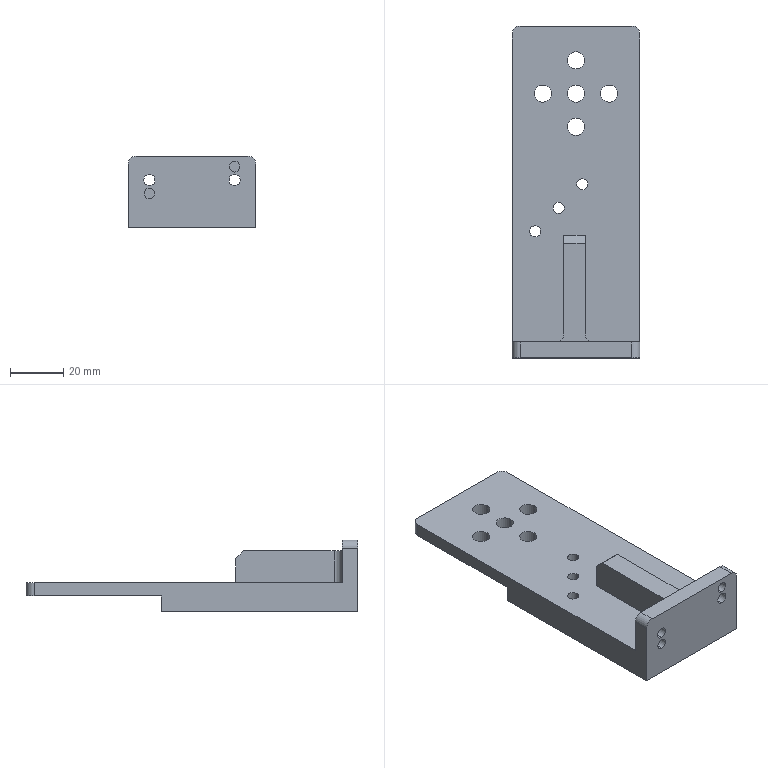NC program | NX | posted with a generic post | part box 48 x 124.7 x 27 mm
Whole program:
N10 G17 G21 G94 G90
(DRILLING_COPY_1_COPY , TOOL : D6A45)
N12 T01 M6
N14 G54
N16 G17 G0 G90 X-16. Y-9.5 B0. C0. S5000 M3
N18 G43 Z30. H1
N20 G94 G81 G98 Z-1. F350. R3.
N22 Y-4.5
N24 X16.
N26 Y0.5
N28 G80
N30 G0 X16. Y0.5 Z30.
N32 M5
(DRILLING_COPY_1_COPY_1_1_COPY_1 , TOOL : 4.2ZT)
N34 T04 M6
N36 G54
N38 G17 G0 G90 X-16. Y-4.5 B0. C0. S2000 M3
N40 G43 Z30. H4
N42 G94 G83 G98 Z-8.762 F200. Q2. R3.
N44 X16.
N46 G80
N48 G0 X16. Y-4.5 Z30.
N50 M5
(HOLE_MILLING , TOOL : D3)
N52 T03 M6
N54 G54
N56 G17 G0 G90 X-16. Y-9.5 B0. C0. S9500 M3
N58 G43 Z30. H3
N60 Z0.5
N62 G94 G3 X-16.2 Y-9.3 R0.2 F1250.
N64 X-16.4 Y-9.5 R0.2
N66 X-16.4 Y-9.5 Z0.3 I0.4 J0.
N68 X-16.4 Y-9.5 Z0.1 I0.4 J0.
N70 X-16.4 Y-9.5 Z-0.1 I0.4 J0.
N72 X-16.4 Y-9.5 Z-0.3 I0.4 J0.
N74 X-16.4 Y-9.5 Z-0.5 I0.4 J0.
N76 X-16.4 Y-9.5 Z-0.7 I0.4 J0.
N78 X-16.4 Y-9.5 Z-0.9 I0.4 J0.
N80 X-16.4 Y-9.5 Z-1.1 I0.4 J0.
N82 X-16.4 Y-9.5 Z-1.3 I0.4 J0.
N84 X-16.4 Y-9.5 Z-1.5 I0.4 J0.
N86 X-16.4 Y-9.5 Z-1.7 I0.4 J0.
N88 X-16.4 Y-9.5 Z-1.9 I0.4 J0.
N90 X-16.4 Y-9.5 Z-2.1 I0.4 J0.
N92 X-16.4 Y-9.5 Z-2.3 I0.4 J0.
N94 X-16.4 Y-9.5 Z-2.5 I0.4 J0.
N96 X-16.4 Y-9.5 Z-2.7 I0.4 J0.
N98 X-16.4 Y-9.5 Z-2.9 I0.4 J0.
N100 X-15.6 Y-9.5 Z-3. I0.4 J0.
N102 X-16. Y-9.1 R0.4
N104 X-15.6 Y-9.5 R-0.4
N106 X-15.8 Y-9.3 R0.2
N108 X-16. Y-9.5 R0.2
N110 G0 Z30.
N112 X16. Y0.5
N114 Z0.5
N116 G3 X15.8 Y0.7 R0.2
N118 X15.6 Y0.5 R0.2
N120 X15.6 Y0.5 Z0.3 I0.4 J0.
N122 X15.6 Y0.5 Z0.1 I0.4 J0.
N124 X15.6 Y0.5 Z-0.1 I0.4 J0.
N126 X15.6 Y0.5 Z-0.3 I0.4 J0.
N128 X15.6 Y0.5 Z-0.5 I0.4 J0.
N130 X15.6 Y0.5 Z-0.7 I0.4 J0.
N132 X15.6 Y0.5 Z-0.9 I0.4 J0.
N134 X15.6 Y0.5 Z-1.1 I0.4 J0.
N136 X15.6 Y0.5 Z-1.3 I0.4 J0.
N138 X15.6 Y0.5 Z-1.5 I0.4 J0.
N140 X15.6 Y0.5 Z-1.7 I0.4 J0.
N142 X15.6 Y0.5 Z-1.9 I0.4 J0.
N144 X15.6 Y0.5 Z-2.1 I0.4 J0.
N146 X15.6 Y0.5 Z-2.3 I0.4 J0.
N148 X15.6 Y0.5 Z-2.5 I0.4 J0.
N150 X15.6 Y0.5 Z-2.7 I0.4 J0.
N152 X15.6 Y0.5 Z-2.9 I0.4 J0.
N154 X16.4 Y0.5 Z-3. I0.4 J0.
N156 X16. Y0.9 R0.4
N158 X16.4 Y0.5 R-0.4
N160 X16.2 Y0.7 R0.2
N162 X16. Y0.5 R0.2
N164 G0 Z30.
N166 M5
(PLANAR_MILL_COPY_COPY_COPY_COPY_COPY_COPY_1_COPY_1_COPY_1_1 , TOOL : D6A45)
N168 T01 M6
N170 G54
N172 G17 G0 G90 X-14.8 Y-9.37 B0. C0. S9500 M3
N174 G43 Z30. H1
N176 Z0.5
N178 G94 G1 Y-9.23 Z0.462 F1250.
N180 X-15.13 Y-8.63 Z0.279
N182 X-15.73 Y-8.3 Z0.096
N184 X-16.27 Z-0.049
N186 X-16.87 Y-8.63 Z-0.233
N188 X-17.2 Y-9.23 Z-0.416
N190 Y-9.77 Z-0.561
N192 X-16.87 Y-10.37 Z-0.744
N194 X-16.27 Y-10.7 Z-0.928
N196 X-16. Z-1.
N198 G3 X-14.8 Y-9.5 R1.2
N200 X-16. Y-10.7 R-1.2
N202 X-15.134 Y-10.2 R1.
N204 G1 Z0.5
N206 G0 Z30.
N208 X-16.068 Y-4.427
N210 Z0.5
N212 G1 Z-1.
N214 X-16.8 Y-3.634
N216 G3 X-17.3 Y-4.5 R1.
N218 X-16. Y-5.8 R1.3
N220 X-17.3 Y-4.5 R-1.3
N222 X-16.8 Y-5.366 R1.
N224 G1 X-16.068 Y-4.573
N226 Z0.5
N228 G0 Z30.
N230 X16.068
N232 Z0.5
N234 G1 Z-1.
N236 X16.8 Y-5.366
N238 G3 X17.3 Y-4.5 R1.
N240 X16. Y-3.2 R1.3
N242 X17.3 Y-4.5 R-1.3
N244 X16.8 Y-3.634 R1.
N246 G1 X16.068 Y-4.427
N248 Z0.5
N250 G0 Z30.
N252 X15.87 Y1.7
N254 Z0.5
N256 G1 X15.73 Z0.462
N258 X15.13 Y1.37 Z0.279
N260 X14.8 Y0.77 Z0.096
N262 Y0.23 Z-0.049
N264 X15.13 Y-0.37 Z-0.233
N266 X15.73 Y-0.7 Z-0.416
N268 X16.27 Z-0.561
N270 X16.87 Y-0.37 Z-0.744
N272 X17.2 Y0.23 Z-0.928
N274 Y0.5 Z-1.
N276 G3 X16. Y1.7 R1.2
N278 X17.2 Y0.5 R-1.2
N280 X16.7 Y1.366 R1.
N282 G1 Z0.5
N284 G0 Z30.
N286 M5
(刀补3 , TOOL : D3)
N288 T03 M6
N290 G54
N292 G17 G0 G90 X-16. Y-9.5 B0. C0. S9500 M3
N294 G43 Z30. H3
N296 Z0.5
N298 G41 G94 G1 X-16.027 Y-9.404 F1000. D3
N300 G3 X-16.45 Y-9.5 R0.222
N302 X-16.45 Y-9.5 Z-0.5 I0.45 J0.
N304 X-16.45 Y-9.5 Z-1.5 I0.45 J0.
N306 X-16.45 Y-9.5 Z-2.5 I0.45 J0.
N308 X-15.55 Y-9.5 Z-3. I0.45 J0.
N310 X-16. Y-9.05 R0.45
N312 X-15.55 Y-9.5 R-0.45
N314 X-15.973 Y-9.404 R0.222
N316 G40
N318 G1 X-16. Y-9.5
N320 G0 Z30.
N322 X16. Y0.5
N324 Z0.5
N326 G41 G1 X15.973 Y0.596
N328 G3 X15.55 Y0.5 R0.222
N330 X15.55 Y0.5 Z-0.5 I0.45 J0.
N332 X15.55 Y0.5 Z-1.5 I0.45 J0.
N334 X15.55 Y0.5 Z-2.5 I0.45 J0.
N336 X16.45 Y0.5 Z-3. I0.45 J0.
N338 X16. Y0.95 R0.45
N340 X16.45 Y0.5 R-0.45
N342 X16.027 Y0.596 R0.222
N344 G40
N346 G1 X16. Y0.5
N348 G0 Z30.
N350 M5
N352 M2